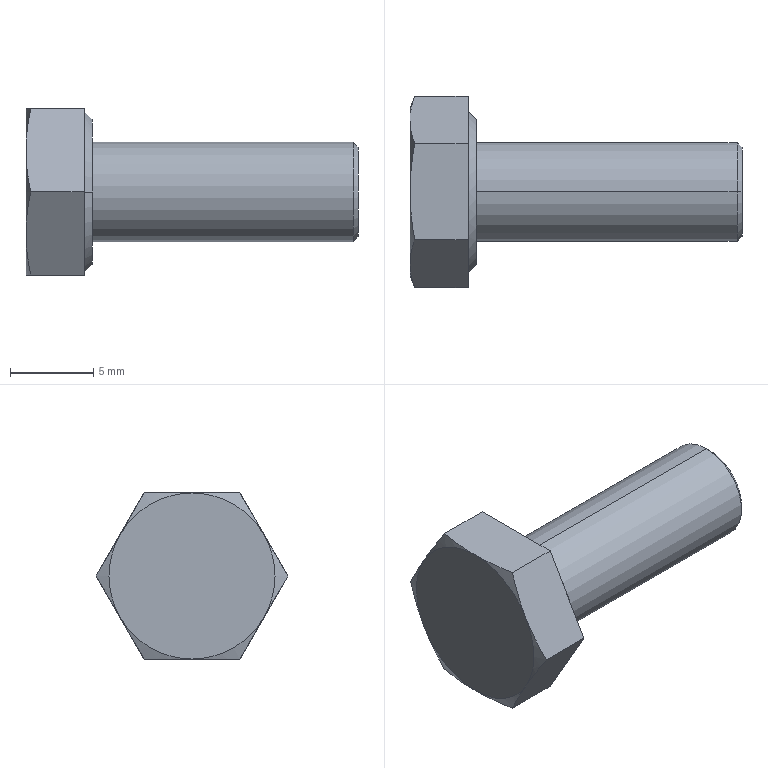Part | STEP file | hex head bolts-full thread grade c gb_GB_FASTENER_BOLT_HHBFTC M6X16-S | 1 solid | 22 faces | box 20 x 11.547 x 10 mm | volume 787.542 mm3 | cone 10 | plane 10 | cylinder 2 | commonest cylinder face diameters 6 x2
STEP:
#1=CARTESIAN_POINT('',(19.7,0.,3.));
#2=VERTEX_POINT('',#1);
#3=CARTESIAN_POINT('',(19.7,0.,-3.));
#4=VERTEX_POINT('',#3);
#5=CARTESIAN_POINT('',(19.7,0.,0.));
#6=DIRECTION('',(-1.,0.,0.));
#7=DIRECTION('',(0.,0.,1.));
#8=AXIS2_PLACEMENT_3D('',#5,#6,#7);
#9=CIRCLE('',#8,3.);
#10=EDGE_CURVE('',#2,#4,#9,.T.);
#11=ORIENTED_EDGE('',*,*,#10,.T.);
#12=CARTESIAN_POINT('',(4.,0.,-3.));
#13=VERTEX_POINT('',#12);
#14=CARTESIAN_POINT('',(20.,0.,-3.));
#15=DIRECTION('',(-1.,0.,0.));
#16=VECTOR('',#15,1000.);
#17=LINE('',#14,#16);
#18=EDGE_CURVE('',#4,#13,#17,.T.);
#19=ORIENTED_EDGE('',*,*,#18,.T.);
#20=CARTESIAN_POINT('',(4.,0.,3.));
#21=VERTEX_POINT('',#20);
#22=CARTESIAN_POINT('',(4.,0.,0.));
#23=DIRECTION('',(1.,0.,0.));
#24=DIRECTION('',(0.,0.,1.));
#25=AXIS2_PLACEMENT_3D('',#22,#23,#24);
#26=CIRCLE('',#25,3.);
#27=EDGE_CURVE('',#13,#21,#26,.T.);
#28=ORIENTED_EDGE('',*,*,#27,.T.);
#29=CARTESIAN_POINT('',(20.,0.,3.));
#30=DIRECTION('',(-1.,0.,0.));
#31=VECTOR('',#30,1000.);
#32=LINE('',#29,#31);
#33=EDGE_CURVE('',#2,#21,#32,.T.);
#34=ORIENTED_EDGE('',*,*,#33,.F.);
#35=EDGE_LOOP('',(#11,#19,#28,#34));
#36=FACE_OUTER_BOUND('',#35,.T.);
#37=CARTESIAN_POINT('',(20.,0.,0.));
#38=DIRECTION('',(-1.,0.,0.));
#39=DIRECTION('',(0.,0.,1.));
#40=AXIS2_PLACEMENT_3D('',#37,#38,#39);
#41=CYLINDRICAL_SURFACE('',#40,3.);
#42=ADVANCED_FACE('',(#36),#41,.T.);
#43=CARTESIAN_POINT('',(20.,0.,2.7));
#44=VERTEX_POINT('',#43);
#45=CARTESIAN_POINT('',(20.,0.,-2.7));
#46=VERTEX_POINT('',#45);
#47=CARTESIAN_POINT('',(20.,0.,0.));
#48=DIRECTION('',(-1.,0.,0.));
#49=DIRECTION('',(0.,0.,1.));
#50=AXIS2_PLACEMENT_3D('',#47,#48,#49);
#51=CIRCLE('',#50,2.7);
#52=EDGE_CURVE('',#44,#46,#51,.T.);
#53=ORIENTED_EDGE('',*,*,#52,.T.);
#54=CARTESIAN_POINT('',(19.7,0.,-3.));
#55=DIRECTION('',(-0.7071,0.,-0.7071));
#56=VECTOR('',#55,1000.);
#57=LINE('',#54,#56);
#58=EDGE_CURVE('',#46,#4,#57,.T.);
#59=ORIENTED_EDGE('',*,*,#58,.T.);
#60=ORIENTED_EDGE('',*,*,#10,.F.);
#61=CARTESIAN_POINT('',(19.7,0.,3.));
#62=DIRECTION('',(-0.7071,0.,0.7071));
#63=VECTOR('',#62,1000.);
#64=LINE('',#61,#63);
#65=EDGE_CURVE('',#44,#2,#64,.T.);
#66=ORIENTED_EDGE('',*,*,#65,.F.);
#67=EDGE_LOOP('',(#53,#59,#60,#66));
#68=FACE_OUTER_BOUND('',#67,.T.);
#69=CARTESIAN_POINT('',(19.7,0.,0.));
#70=DIRECTION('',(-1.,0.,0.));
#71=DIRECTION('',(0.,0.,1.));
#72=AXIS2_PLACEMENT_3D('',#69,#70,#71);
#73=CONICAL_SURFACE('',#72,3.,0.7854);
#74=ADVANCED_FACE('',(#68),#73,.T.);
#75=CARTESIAN_POINT('',(4.,-4.37,0.));
#76=VERTEX_POINT('',#75);
#77=CARTESIAN_POINT('',(4.,4.37,0.));
#78=VERTEX_POINT('',#77);
#79=CARTESIAN_POINT('',(4.,0.,0.));
#80=DIRECTION('',(-1.,0.,0.));
#81=DIRECTION('',(0.,-1.,0.));
#82=AXIS2_PLACEMENT_3D('',#79,#80,#81);
#83=CIRCLE('',#82,4.37);
#84=EDGE_CURVE('',#76,#78,#83,.T.);
#85=ORIENTED_EDGE('',*,*,#84,.T.);
#86=CARTESIAN_POINT('',(3.5,4.87,0.));
#87=VERTEX_POINT('',#86);
#88=CARTESIAN_POINT('',(3.5,4.87,0.));
#89=DIRECTION('',(-0.7071,0.7071,0.));
#90=VECTOR('',#89,1000.);
#91=LINE('',#88,#90);
#92=EDGE_CURVE('',#78,#87,#91,.T.);
#93=ORIENTED_EDGE('',*,*,#92,.T.);
#94=CARTESIAN_POINT('',(3.5,-4.87,0.));
#95=VERTEX_POINT('',#94);
#96=CARTESIAN_POINT('',(3.5,0.,0.));
#97=DIRECTION('',(1.,0.,0.));
#98=DIRECTION('',(0.,-1.,0.));
#99=AXIS2_PLACEMENT_3D('',#96,#97,#98);
#100=CIRCLE('',#99,4.87);
#101=EDGE_CURVE('',#87,#95,#100,.T.);
#102=ORIENTED_EDGE('',*,*,#101,.T.);
#103=CARTESIAN_POINT('',(3.5,-4.87,0.));
#104=DIRECTION('',(-0.7071,-0.7071,0.));
#105=VECTOR('',#104,1000.);
#106=LINE('',#103,#105);
#107=EDGE_CURVE('',#76,#95,#106,.T.);
#108=ORIENTED_EDGE('',*,*,#107,.F.);
#109=EDGE_LOOP('',(#85,#93,#102,#108));
#110=FACE_OUTER_BOUND('',#109,.T.);
#111=CARTESIAN_POINT('',(3.5,0.,0.));
#112=DIRECTION('',(-1.,0.,0.));
#113=DIRECTION('',(0.,-1.,0.));
#114=AXIS2_PLACEMENT_3D('',#111,#112,#113);
#115=CONICAL_SURFACE('',#114,4.87,0.7854);
#116=ADVANCED_FACE('',(#110),#115,.T.);
#117=ORIENTED_EDGE('',*,*,#18,.F.);
#118=CARTESIAN_POINT('',(19.7,0.,0.));
#119=DIRECTION('',(-1.,0.,0.));
#120=DIRECTION('',(0.,0.,1.));
#121=AXIS2_PLACEMENT_3D('',#118,#119,#120);
#122=CIRCLE('',#121,3.);
#123=EDGE_CURVE('',#4,#2,#122,.T.);
#124=ORIENTED_EDGE('',*,*,#123,.T.);
#125=ORIENTED_EDGE('',*,*,#33,.T.);
#126=CARTESIAN_POINT('',(4.,0.,0.));
#127=DIRECTION('',(1.,0.,0.));
#128=DIRECTION('',(0.,0.,1.));
#129=AXIS2_PLACEMENT_3D('',#126,#127,#128);
#130=CIRCLE('',#129,3.);
#131=EDGE_CURVE('',#21,#13,#130,.T.);
#132=ORIENTED_EDGE('',*,*,#131,.T.);
#133=EDGE_LOOP('',(#117,#124,#125,#132));
#134=FACE_OUTER_BOUND('',#133,.T.);
#135=CARTESIAN_POINT('',(20.,0.,0.));
#136=DIRECTION('',(-1.,0.,0.));
#137=DIRECTION('',(0.,0.,1.));
#138=AXIS2_PLACEMENT_3D('',#135,#136,#137);
#139=CYLINDRICAL_SURFACE('',#138,3.);
#140=ADVANCED_FACE('',(#134),#139,.T.);
#141=ORIENTED_EDGE('',*,*,#131,.F.);
#142=ORIENTED_EDGE('',*,*,#27,.F.);
#143=EDGE_LOOP('',(#141,#142));
#144=FACE_BOUND('',#143,.T.);
#145=ORIENTED_EDGE('',*,*,#84,.F.);
#146=CARTESIAN_POINT('',(4.,0.,0.));
#147=DIRECTION('',(-1.,0.,0.));
#148=DIRECTION('',(0.,-1.,0.));
#149=AXIS2_PLACEMENT_3D('',#146,#147,#148);
#150=CIRCLE('',#149,4.37);
#151=EDGE_CURVE('',#78,#76,#150,.T.);
#152=ORIENTED_EDGE('',*,*,#151,.F.);
#153=EDGE_LOOP('',(#145,#152));
#154=FACE_OUTER_BOUND('',#153,.T.);
#155=CARTESIAN_POINT('',(4.,0.,10.));
#156=DIRECTION('',(-1.,0.,0.));
#157=DIRECTION('',(0.,0.,1.));
#158=AXIS2_PLACEMENT_3D('',#155,#156,#157);
#159=PLANE('',#158);
#160=ADVANCED_FACE('',(#144,#154),#159,.F.);
#161=ORIENTED_EDGE('',*,*,#58,.F.);
#162=CARTESIAN_POINT('',(20.,0.,0.));
#163=DIRECTION('',(-1.,0.,0.));
#164=DIRECTION('',(0.,0.,1.));
#165=AXIS2_PLACEMENT_3D('',#162,#163,#164);
#166=CIRCLE('',#165,2.7);
#167=EDGE_CURVE('',#46,#44,#166,.T.);
#168=ORIENTED_EDGE('',*,*,#167,.T.);
#169=ORIENTED_EDGE('',*,*,#65,.T.);
#170=ORIENTED_EDGE('',*,*,#123,.F.);
#171=EDGE_LOOP('',(#161,#168,#169,#170));
#172=FACE_OUTER_BOUND('',#171,.T.);
#173=CARTESIAN_POINT('',(19.7,0.,0.));
#174=DIRECTION('',(-1.,0.,0.));
#175=DIRECTION('',(0.,0.,1.));
#176=AXIS2_PLACEMENT_3D('',#173,#174,#175);
#177=CONICAL_SURFACE('',#176,3.,0.7854);
#178=ADVANCED_FACE('',(#172),#177,.T.);
#179=ORIENTED_EDGE('',*,*,#92,.F.);
#180=ORIENTED_EDGE('',*,*,#151,.T.);
#181=ORIENTED_EDGE('',*,*,#107,.T.);
#182=CARTESIAN_POINT('',(3.5,0.,0.));
#183=DIRECTION('',(1.,0.,0.));
#184=DIRECTION('',(0.,-1.,0.));
#185=AXIS2_PLACEMENT_3D('',#182,#183,#184);
#186=CIRCLE('',#185,4.87);
#187=EDGE_CURVE('',#95,#87,#186,.T.);
#188=ORIENTED_EDGE('',*,*,#187,.T.);
#189=EDGE_LOOP('',(#179,#180,#181,#188));
#190=FACE_OUTER_BOUND('',#189,.T.);
#191=CARTESIAN_POINT('',(3.5,0.,0.));
#192=DIRECTION('',(-1.,0.,0.));
#193=DIRECTION('',(0.,-1.,0.));
#194=AXIS2_PLACEMENT_3D('',#191,#192,#193);
#195=CONICAL_SURFACE('',#194,4.87,0.7854);
#196=ADVANCED_FACE('',(#190),#195,.T.);
#197=ORIENTED_EDGE('',*,*,#52,.F.);
#198=ORIENTED_EDGE('',*,*,#167,.F.);
#199=EDGE_LOOP('',(#197,#198));
#200=FACE_OUTER_BOUND('',#199,.T.);
#201=CARTESIAN_POINT('',(20.,0.,0.));
#202=DIRECTION('',(1.,0.,0.));
#203=DIRECTION('',(0.,0.,-1.));
#204=AXIS2_PLACEMENT_3D('',#201,#202,#203);
#205=PLANE('',#204);
#206=ADVANCED_FACE('',(#200),#205,.T.);
#207=CARTESIAN_POINT('',(3.5,5.774,0.));
#208=VERTEX_POINT('',#207);
#209=CARTESIAN_POINT('',(3.5,2.887,5.));
#210=VERTEX_POINT('',#209);
#211=CARTESIAN_POINT('',(3.5,5.774,0.));
#212=DIRECTION('',(0.,-0.5,0.866));
#213=VECTOR('',#212,1000.);
#214=LINE('',#211,#213);
#215=EDGE_CURVE('',#208,#210,#214,.T.);
#216=ORIENTED_EDGE('',*,*,#215,.T.);
#217=CARTESIAN_POINT('',(3.5,-2.887,5.));
#218=VERTEX_POINT('',#217);
#219=CARTESIAN_POINT('',(3.5,4.87,5.));
#220=DIRECTION('',(0.,-1.,0.));
#221=VECTOR('',#220,1000.);
#222=LINE('',#219,#221);
#223=EDGE_CURVE('',#210,#218,#222,.T.);
#224=ORIENTED_EDGE('',*,*,#223,.T.);
#225=CARTESIAN_POINT('',(3.5,-5.774,0.));
#226=VERTEX_POINT('',#225);
#227=CARTESIAN_POINT('',(3.5,-2.887,5.));
#228=DIRECTION('',(0.,-0.5,-0.866));
#229=VECTOR('',#228,1000.);
#230=LINE('',#227,#229);
#231=EDGE_CURVE('',#218,#226,#230,.T.);
#232=ORIENTED_EDGE('',*,*,#231,.T.);
#233=CARTESIAN_POINT('',(3.5,-2.887,-5.));
#234=VERTEX_POINT('',#233);
#235=CARTESIAN_POINT('',(3.5,-5.774,0.));
#236=DIRECTION('',(0.,0.5,-0.866));
#237=VECTOR('',#236,1000.);
#238=LINE('',#235,#237);
#239=EDGE_CURVE('',#226,#234,#238,.T.);
#240=ORIENTED_EDGE('',*,*,#239,.T.);
#241=CARTESIAN_POINT('',(3.5,2.887,-5.));
#242=VERTEX_POINT('',#241);
#243=CARTESIAN_POINT('',(3.5,4.87,-5.));
#244=DIRECTION('',(0.,1.,0.));
#245=VECTOR('',#244,1000.);
#246=LINE('',#243,#245);
#247=EDGE_CURVE('',#234,#242,#246,.T.);
#248=ORIENTED_EDGE('',*,*,#247,.T.);
#249=CARTESIAN_POINT('',(3.5,2.887,-5.));
#250=DIRECTION('',(0.,0.5,0.866));
#251=VECTOR('',#250,1000.);
#252=LINE('',#249,#251);
#253=EDGE_CURVE('',#242,#208,#252,.T.);
#254=ORIENTED_EDGE('',*,*,#253,.T.);
#255=EDGE_LOOP('',(#216,#224,#232,#240,#248,#254));
#256=FACE_OUTER_BOUND('',#255,.T.);
#257=ORIENTED_EDGE('',*,*,#187,.F.);
#258=ORIENTED_EDGE('',*,*,#101,.F.);
#259=EDGE_LOOP('',(#257,#258));
#260=FACE_BOUND('',#259,.T.);
#261=CARTESIAN_POINT('',(3.5,4.87,0.));
#262=DIRECTION('',(1.,0.,0.));
#263=DIRECTION('',(0.,0.,-1.));
#264=AXIS2_PLACEMENT_3D('',#261,#262,#263);
#265=PLANE('',#264);
#266=ADVANCED_FACE('',(#256,#260),#265,.T.);
#267=CARTESIAN_POINT('',(0.2815,-2.887,5.));
#268=VERTEX_POINT('',#267);
#269=CARTESIAN_POINT('',(4.,-2.887,5.));
#270=DIRECTION('',(-1.,0.,0.));
#271=VECTOR('',#270,1000.);
#272=LINE('',#269,#271);
#273=EDGE_CURVE('',#218,#268,#272,.T.);
#274=ORIENTED_EDGE('',*,*,#273,.F.);
#275=ORIENTED_EDGE('',*,*,#223,.F.);
#276=CARTESIAN_POINT('',(0.2815,2.887,5.));
#277=VERTEX_POINT('',#276);
#278=CARTESIAN_POINT('',(4.,2.887,5.));
#279=DIRECTION('',(1.,0.,0.));
#280=VECTOR('',#279,1000.);
#281=LINE('',#278,#280);
#282=EDGE_CURVE('',#277,#210,#281,.T.);
#283=ORIENTED_EDGE('',*,*,#282,.F.);
#284=CARTESIAN_POINT('',(0.,0.,5.));
#285=VERTEX_POINT('',#284);
#286=CARTESIAN_POINT('',(0.,0.,5.));
#287=CARTESIAN_POINT('',(0.,0.9714,5.));
#288=CARTESIAN_POINT('',(0.1078,1.932,5.));
#289=CARTESIAN_POINT('',(0.2815,2.887,5.));
#290=B_SPLINE_CURVE_WITH_KNOTS('',3,(#286,#287,#288,#289),.UNSPECIFIED.,.F.,.F.,(4,4),(0.,0.0029),.UNSPECIFIED.);
#291=EDGE_CURVE('',#285,#277,#290,.T.);
#292=ORIENTED_EDGE('',*,*,#291,.F.);
#293=CARTESIAN_POINT('',(0.2815,-2.887,5.));
#294=CARTESIAN_POINT('',(0.1078,-1.932,5.));
#295=CARTESIAN_POINT('',(0.,-0.9714,5.));
#296=CARTESIAN_POINT('',(0.,0.,5.));
#297=B_SPLINE_CURVE_WITH_KNOTS('',3,(#293,#294,#295,#296),.UNSPECIFIED.,.F.,.F.,(4,4),(0.,0.0029),.UNSPECIFIED.);
#298=EDGE_CURVE('',#268,#285,#297,.T.);
#299=ORIENTED_EDGE('',*,*,#298,.F.);
#300=EDGE_LOOP('',(#274,#275,#283,#292,#299));
#301=FACE_OUTER_BOUND('',#300,.T.);
#302=CARTESIAN_POINT('',(4.,2.887,5.));
#303=DIRECTION('',(0.,0.,-1.));
#304=DIRECTION('',(-1.,0.,0.));
#305=AXIS2_PLACEMENT_3D('',#302,#303,#304);
#306=PLANE('',#305);
#307=ADVANCED_FACE('',(#301),#306,.F.);
#308=ORIENTED_EDGE('',*,*,#282,.T.);
#309=ORIENTED_EDGE('',*,*,#215,.F.);
#310=CARTESIAN_POINT('',(0.2815,5.774,0.));
#311=VERTEX_POINT('',#310);
#312=CARTESIAN_POINT('',(4.,5.774,0.));
#313=DIRECTION('',(1.,0.,0.));
#314=VECTOR('',#313,1000.);
#315=LINE('',#312,#314);
#316=EDGE_CURVE('',#311,#208,#315,.T.);
#317=ORIENTED_EDGE('',*,*,#316,.F.);
#318=CARTESIAN_POINT('',(0.,4.33,2.5));
#319=VERTEX_POINT('',#318);
#320=CARTESIAN_POINT('',(0.,4.33,2.5));
#321=CARTESIAN_POINT('',(0.,4.816,1.659));
#322=CARTESIAN_POINT('',(0.1078,5.296,0.8266));
#323=CARTESIAN_POINT('',(0.2815,5.774,0.));
#324=B_SPLINE_CURVE_WITH_KNOTS('',3,(#320,#321,#322,#323),.UNSPECIFIED.,.F.,.F.,(4,4),(0.,0.0029),.UNSPECIFIED.);
#325=EDGE_CURVE('',#319,#311,#324,.T.);
#326=ORIENTED_EDGE('',*,*,#325,.F.);
#327=CARTESIAN_POINT('',(0.2815,2.887,5.));
#328=CARTESIAN_POINT('',(0.1078,3.364,4.173));
#329=CARTESIAN_POINT('',(0.,3.844,3.341));
#330=CARTESIAN_POINT('',(0.,4.33,2.5));
#331=B_SPLINE_CURVE_WITH_KNOTS('',3,(#327,#328,#329,#330),.UNSPECIFIED.,.F.,.F.,(4,4),(0.,0.0029),.UNSPECIFIED.);
#332=EDGE_CURVE('',#277,#319,#331,.T.);
#333=ORIENTED_EDGE('',*,*,#332,.F.);
#334=EDGE_LOOP('',(#308,#309,#317,#326,#333));
#335=FACE_OUTER_BOUND('',#334,.T.);
#336=CARTESIAN_POINT('',(4.,5.774,0.));
#337=DIRECTION('',(0.,-0.866,-0.5));
#338=DIRECTION('',(0.,0.5,-0.866));
#339=AXIS2_PLACEMENT_3D('',#336,#337,#338);
#340=PLANE('',#339);
#341=ADVANCED_FACE('',(#335),#340,.F.);
#342=ORIENTED_EDGE('',*,*,#316,.T.);
#343=ORIENTED_EDGE('',*,*,#253,.F.);
#344=CARTESIAN_POINT('',(0.2815,2.887,-5.));
#345=VERTEX_POINT('',#344);
#346=CARTESIAN_POINT('',(4.,2.887,-5.));
#347=DIRECTION('',(1.,0.,0.));
#348=VECTOR('',#347,1000.);
#349=LINE('',#346,#348);
#350=EDGE_CURVE('',#345,#242,#349,.T.);
#351=ORIENTED_EDGE('',*,*,#350,.F.);
#352=CARTESIAN_POINT('',(0.,4.33,-2.5));
#353=VERTEX_POINT('',#352);
#354=CARTESIAN_POINT('',(0.,4.33,-2.5));
#355=CARTESIAN_POINT('',(0.,3.844,-3.341));
#356=CARTESIAN_POINT('',(0.1078,3.364,-4.173));
#357=CARTESIAN_POINT('',(0.2815,2.887,-5.));
#358=B_SPLINE_CURVE_WITH_KNOTS('',3,(#354,#355,#356,#357),.UNSPECIFIED.,.F.,.F.,(4,4),(0.,0.0029),.UNSPECIFIED.);
#359=EDGE_CURVE('',#353,#345,#358,.T.);
#360=ORIENTED_EDGE('',*,*,#359,.F.);
#361=CARTESIAN_POINT('',(0.2815,5.774,0.));
#362=CARTESIAN_POINT('',(0.1078,5.296,-0.8266));
#363=CARTESIAN_POINT('',(0.,4.816,-1.659));
#364=CARTESIAN_POINT('',(0.,4.33,-2.5));
#365=B_SPLINE_CURVE_WITH_KNOTS('',3,(#361,#362,#363,#364),.UNSPECIFIED.,.F.,.F.,(4,4),(0.,0.0029),.UNSPECIFIED.);
#366=EDGE_CURVE('',#311,#353,#365,.T.);
#367=ORIENTED_EDGE('',*,*,#366,.F.);
#368=EDGE_LOOP('',(#342,#343,#351,#360,#367));
#369=FACE_OUTER_BOUND('',#368,.T.);
#370=CARTESIAN_POINT('',(4.,2.887,-5.));
#371=DIRECTION('',(0.,-0.866,0.5));
#372=DIRECTION('',(0.,-0.5,-0.866));
#373=AXIS2_PLACEMENT_3D('',#370,#371,#372);
#374=PLANE('',#373);
#375=ADVANCED_FACE('',(#369),#374,.F.);
#376=ORIENTED_EDGE('',*,*,#350,.T.);
#377=ORIENTED_EDGE('',*,*,#247,.F.);
#378=CARTESIAN_POINT('',(0.2815,-2.887,-5.));
#379=VERTEX_POINT('',#378);
#380=CARTESIAN_POINT('',(4.,-2.887,-5.));
#381=DIRECTION('',(1.,0.,0.));
#382=VECTOR('',#381,1000.);
#383=LINE('',#380,#382);
#384=EDGE_CURVE('',#379,#234,#383,.T.);
#385=ORIENTED_EDGE('',*,*,#384,.F.);
#386=CARTESIAN_POINT('',(0.,0.,-5.));
#387=VERTEX_POINT('',#386);
#388=CARTESIAN_POINT('',(0.,0.,-5.));
#389=CARTESIAN_POINT('',(0.,-0.9714,-5.));
#390=CARTESIAN_POINT('',(0.1078,-1.932,-5.));
#391=CARTESIAN_POINT('',(0.2815,-2.887,-5.));
#392=B_SPLINE_CURVE_WITH_KNOTS('',3,(#388,#389,#390,#391),.UNSPECIFIED.,.F.,.F.,(4,4),(0.,0.0029),.UNSPECIFIED.);
#393=EDGE_CURVE('',#387,#379,#392,.T.);
#394=ORIENTED_EDGE('',*,*,#393,.F.);
#395=CARTESIAN_POINT('',(0.2815,2.887,-5.));
#396=CARTESIAN_POINT('',(0.1078,1.932,-5.));
#397=CARTESIAN_POINT('',(0.,0.9714,-5.));
#398=CARTESIAN_POINT('',(0.,0.,-5.));
#399=B_SPLINE_CURVE_WITH_KNOTS('',3,(#395,#396,#397,#398),.UNSPECIFIED.,.F.,.F.,(4,4),(0.,0.0029),.UNSPECIFIED.);
#400=EDGE_CURVE('',#345,#387,#399,.T.);
#401=ORIENTED_EDGE('',*,*,#400,.F.);
#402=EDGE_LOOP('',(#376,#377,#385,#394,#401));
#403=FACE_OUTER_BOUND('',#402,.T.);
#404=CARTESIAN_POINT('',(4.,-2.887,-5.));
#405=DIRECTION('',(0.,0.,1.));
#406=DIRECTION('',(1.,0.,0.));
#407=AXIS2_PLACEMENT_3D('',#404,#405,#406);
#408=PLANE('',#407);
#409=ADVANCED_FACE('',(#403),#408,.F.);
#410=ORIENTED_EDGE('',*,*,#384,.T.);
#411=ORIENTED_EDGE('',*,*,#239,.F.);
#412=CARTESIAN_POINT('',(0.2815,-5.774,0.));
#413=VERTEX_POINT('',#412);
#414=CARTESIAN_POINT('',(4.,-5.774,0.));
#415=DIRECTION('',(1.,0.,0.));
#416=VECTOR('',#415,1000.);
#417=LINE('',#414,#416);
#418=EDGE_CURVE('',#413,#226,#417,.T.);
#419=ORIENTED_EDGE('',*,*,#418,.F.);
#420=CARTESIAN_POINT('',(0.,-4.33,-2.5));
#421=VERTEX_POINT('',#420);
#422=CARTESIAN_POINT('',(0.,-4.33,-2.5));
#423=CARTESIAN_POINT('',(0.,-4.816,-1.659));
#424=CARTESIAN_POINT('',(0.1078,-5.296,-0.8266));
#425=CARTESIAN_POINT('',(0.2815,-5.774,0.));
#426=B_SPLINE_CURVE_WITH_KNOTS('',3,(#422,#423,#424,#425),.UNSPECIFIED.,.F.,.F.,(4,4),(0.,0.0029),.UNSPECIFIED.);
#427=EDGE_CURVE('',#421,#413,#426,.T.);
#428=ORIENTED_EDGE('',*,*,#427,.F.);
#429=CARTESIAN_POINT('',(0.2815,-2.887,-5.));
#430=CARTESIAN_POINT('',(0.1078,-3.364,-4.173));
#431=CARTESIAN_POINT('',(0.,-3.844,-3.341));
#432=CARTESIAN_POINT('',(0.,-4.33,-2.5));
#433=B_SPLINE_CURVE_WITH_KNOTS('',3,(#429,#430,#431,#432),.UNSPECIFIED.,.F.,.F.,(4,4),(0.,0.0029),.UNSPECIFIED.);
#434=EDGE_CURVE('',#379,#421,#433,.T.);
#435=ORIENTED_EDGE('',*,*,#434,.F.);
#436=EDGE_LOOP('',(#410,#411,#419,#428,#435));
#437=FACE_OUTER_BOUND('',#436,.T.);
#438=CARTESIAN_POINT('',(4.,-5.774,0.));
#439=DIRECTION('',(0.,0.866,0.5));
#440=DIRECTION('',(0.,-0.5,0.866));
#441=AXIS2_PLACEMENT_3D('',#438,#439,#440);
#442=PLANE('',#441);
#443=ADVANCED_FACE('',(#437),#442,.F.);
#444=ORIENTED_EDGE('',*,*,#418,.T.);
#445=ORIENTED_EDGE('',*,*,#231,.F.);
#446=ORIENTED_EDGE('',*,*,#273,.T.);
#447=CARTESIAN_POINT('',(0.,-4.33,2.5));
#448=VERTEX_POINT('',#447);
#449=CARTESIAN_POINT('',(0.,-4.33,2.5));
#450=CARTESIAN_POINT('',(0.,-3.844,3.341));
#451=CARTESIAN_POINT('',(0.1078,-3.364,4.173));
#452=CARTESIAN_POINT('',(0.2815,-2.887,5.));
#453=B_SPLINE_CURVE_WITH_KNOTS('',3,(#449,#450,#451,#452),.UNSPECIFIED.,.F.,.F.,(4,4),(0.,0.0029),.UNSPECIFIED.);
#454=EDGE_CURVE('',#448,#268,#453,.T.);
#455=ORIENTED_EDGE('',*,*,#454,.F.);
#456=CARTESIAN_POINT('',(0.2815,-5.774,0.));
#457=CARTESIAN_POINT('',(0.1078,-5.296,0.8266));
#458=CARTESIAN_POINT('',(0.,-4.816,1.659));
#459=CARTESIAN_POINT('',(0.,-4.33,2.5));
#460=B_SPLINE_CURVE_WITH_KNOTS('',3,(#456,#457,#458,#459),.UNSPECIFIED.,.F.,.F.,(4,4),(0.,0.0029),.UNSPECIFIED.);
#461=EDGE_CURVE('',#413,#448,#460,.T.);
#462=ORIENTED_EDGE('',*,*,#461,.F.);
#463=EDGE_LOOP('',(#444,#445,#446,#455,#462));
#464=FACE_OUTER_BOUND('',#463,.T.);
#465=CARTESIAN_POINT('',(4.,-2.887,5.));
#466=DIRECTION('',(0.,0.866,-0.5));
#467=DIRECTION('',(0.,0.5,0.866));
#468=AXIS2_PLACEMENT_3D('',#465,#466,#467);
#469=PLANE('',#468);
#470=ADVANCED_FACE('',(#464),#469,.F.);
#471=ORIENTED_EDGE('',*,*,#298,.T.);
#472=CARTESIAN_POINT('',(0.,0.,0.));
#473=DIRECTION('',(1.,0.,0.));
#474=DIRECTION('',(0.,0.,-1.));
#475=AXIS2_PLACEMENT_3D('',#472,#473,#474);
#476=CIRCLE('',#475,5.);
#477=EDGE_CURVE('',#285,#448,#476,.T.);
#478=ORIENTED_EDGE('',*,*,#477,.T.);
#479=ORIENTED_EDGE('',*,*,#454,.T.);
#480=EDGE_LOOP('',(#471,#478,#479));
#481=FACE_OUTER_BOUND('',#480,.T.);
#482=CARTESIAN_POINT('',(0.2832,0.,0.));
#483=DIRECTION('',(1.,0.,0.));
#484=DIRECTION('',(0.,0.,-1.));
#485=AXIS2_PLACEMENT_3D('',#482,#483,#484);
#486=CONICAL_SURFACE('',#485,5.778,1.222);
#487=ADVANCED_FACE('',(#481),#486,.T.);
#488=CARTESIAN_POINT('',(0.,0.,0.));
#489=DIRECTION('',(1.,0.,0.));
#490=DIRECTION('',(0.,0.,-1.));
#491=AXIS2_PLACEMENT_3D('',#488,#489,#490);
#492=CIRCLE('',#491,5.);
#493=EDGE_CURVE('',#319,#285,#492,.T.);
#494=ORIENTED_EDGE('',*,*,#493,.T.);
#495=ORIENTED_EDGE('',*,*,#291,.T.);
#496=ORIENTED_EDGE('',*,*,#332,.T.);
#497=EDGE_LOOP('',(#494,#495,#496));
#498=FACE_OUTER_BOUND('',#497,.T.);
#499=CARTESIAN_POINT('',(0.2832,0.,0.));
#500=DIRECTION('',(1.,0.,0.));
#501=DIRECTION('',(0.,0.,-1.));
#502=AXIS2_PLACEMENT_3D('',#499,#500,#501);
#503=CONICAL_SURFACE('',#502,5.778,1.222);
#504=ADVANCED_FACE('',(#498),#503,.T.);
#505=CARTESIAN_POINT('',(0.,0.,0.));
#506=DIRECTION('',(1.,0.,0.));
#507=DIRECTION('',(0.,0.,-1.));
#508=AXIS2_PLACEMENT_3D('',#505,#506,#507);
#509=CIRCLE('',#508,5.);
#510=EDGE_CURVE('',#353,#319,#509,.T.);
#511=ORIENTED_EDGE('',*,*,#510,.T.);
#512=ORIENTED_EDGE('',*,*,#325,.T.);
#513=ORIENTED_EDGE('',*,*,#366,.T.);
#514=EDGE_LOOP('',(#511,#512,#513));
#515=FACE_OUTER_BOUND('',#514,.T.);
#516=CARTESIAN_POINT('',(0.2832,0.,0.));
#517=DIRECTION('',(1.,0.,0.));
#518=DIRECTION('',(0.,0.,-1.));
#519=AXIS2_PLACEMENT_3D('',#516,#517,#518);
#520=CONICAL_SURFACE('',#519,5.778,1.222);
#521=ADVANCED_FACE('',(#515),#520,.T.);
#522=CARTESIAN_POINT('',(0.,0.,0.));
#523=DIRECTION('',(1.,0.,0.));
#524=DIRECTION('',(0.,0.,-1.));
#525=AXIS2_PLACEMENT_3D('',#522,#523,#524);
#526=CIRCLE('',#525,5.);
#527=EDGE_CURVE('',#387,#353,#526,.T.);
#528=ORIENTED_EDGE('',*,*,#527,.T.);
#529=ORIENTED_EDGE('',*,*,#359,.T.);
#530=ORIENTED_EDGE('',*,*,#400,.T.);
#531=EDGE_LOOP('',(#528,#529,#530));
#532=FACE_OUTER_BOUND('',#531,.T.);
#533=CARTESIAN_POINT('',(0.2832,0.,0.));
#534=DIRECTION('',(1.,0.,0.));
#535=DIRECTION('',(0.,0.,-1.));
#536=AXIS2_PLACEMENT_3D('',#533,#534,#535);
#537=CONICAL_SURFACE('',#536,5.778,1.222);
#538=ADVANCED_FACE('',(#532),#537,.T.);
#539=ORIENTED_EDGE('',*,*,#434,.T.);
#540=CARTESIAN_POINT('',(0.,0.,0.));
#541=DIRECTION('',(1.,0.,0.));
#542=DIRECTION('',(0.,0.,-1.));
#543=AXIS2_PLACEMENT_3D('',#540,#541,#542);
#544=CIRCLE('',#543,5.);
#545=EDGE_CURVE('',#421,#387,#544,.T.);
#546=ORIENTED_EDGE('',*,*,#545,.T.);
#547=ORIENTED_EDGE('',*,*,#393,.T.);
#548=EDGE_LOOP('',(#539,#546,#547));
#549=FACE_OUTER_BOUND('',#548,.T.);
#550=CARTESIAN_POINT('',(0.2832,0.,0.));
#551=DIRECTION('',(1.,0.,0.));
#552=DIRECTION('',(0.,0.,-1.));
#553=AXIS2_PLACEMENT_3D('',#550,#551,#552);
#554=CONICAL_SURFACE('',#553,5.778,1.222);
#555=ADVANCED_FACE('',(#549),#554,.T.);
#556=ORIENTED_EDGE('',*,*,#461,.T.);
#557=CARTESIAN_POINT('',(0.,0.,0.));
#558=DIRECTION('',(1.,0.,0.));
#559=DIRECTION('',(0.,0.,-1.));
#560=AXIS2_PLACEMENT_3D('',#557,#558,#559);
#561=CIRCLE('',#560,5.);
#562=EDGE_CURVE('',#448,#421,#561,.T.);
#563=ORIENTED_EDGE('',*,*,#562,.T.);
#564=ORIENTED_EDGE('',*,*,#427,.T.);
#565=EDGE_LOOP('',(#556,#563,#564));
#566=FACE_OUTER_BOUND('',#565,.T.);
#567=CARTESIAN_POINT('',(0.2832,0.,0.));
#568=DIRECTION('',(1.,0.,0.));
#569=DIRECTION('',(0.,0.,-1.));
#570=AXIS2_PLACEMENT_3D('',#567,#568,#569);
#571=CONICAL_SURFACE('',#570,5.778,1.222);
#572=ADVANCED_FACE('',(#566),#571,.T.);
#573=ORIENTED_EDGE('',*,*,#545,.F.);
#574=ORIENTED_EDGE('',*,*,#562,.F.);
#575=ORIENTED_EDGE('',*,*,#477,.F.);
#576=ORIENTED_EDGE('',*,*,#493,.F.);
#577=ORIENTED_EDGE('',*,*,#510,.F.);
#578=ORIENTED_EDGE('',*,*,#527,.F.);
#579=EDGE_LOOP('',(#573,#574,#575,#576,#577,#578));
#580=FACE_OUTER_BOUND('',#579,.T.);
#581=CARTESIAN_POINT('',(0.,0.,10.));
#582=DIRECTION('',(-1.,0.,0.));
#583=DIRECTION('',(0.,0.,1.));
#584=AXIS2_PLACEMENT_3D('',#581,#582,#583);
#585=PLANE('',#584);
#586=ADVANCED_FACE('',(#580),#585,.T.);
#587=CLOSED_SHELL('',(#42,#74,#116,#140,#160,#178,#196,#206,#266,#307,#341,#375,#409,#443,#470,#487,#504,#521,#538,#555,#572,#586));
#588=MANIFOLD_SOLID_BREP('',#587);
#589=CARTESIAN_POINT('',(0.,0.,0.));
#590=DIRECTION('',(0.,0.,1.));
#591=DIRECTION('',(1.,0.,0.));
#592=AXIS2_PLACEMENT_3D('',#589,#590,#591);
#593=(LENGTH_UNIT()NAMED_UNIT(*)SI_UNIT(.MILLI.,.METRE.));
#594=UNCERTAINTY_MEASURE_WITH_UNIT(LENGTH_MEASURE(0.00001),#593,'','');
#595=(NAMED_UNIT(*)PLANE_ANGLE_UNIT()SI_UNIT($,.RADIAN.));
#596=(NAMED_UNIT(*)SI_UNIT($,.STERADIAN.)SOLID_ANGLE_UNIT());
#597=(GEOMETRIC_REPRESENTATION_CONTEXT(3)GLOBAL_UNCERTAINTY_ASSIGNED_CONTEXT((#594))GLOBAL_UNIT_ASSIGNED_CONTEXT((#593,#595,#596))REPRESENTATION_CONTEXT('',''));
#598=ADVANCED_BREP_SHAPE_REPRESENTATION('',(#588,#592),#597);